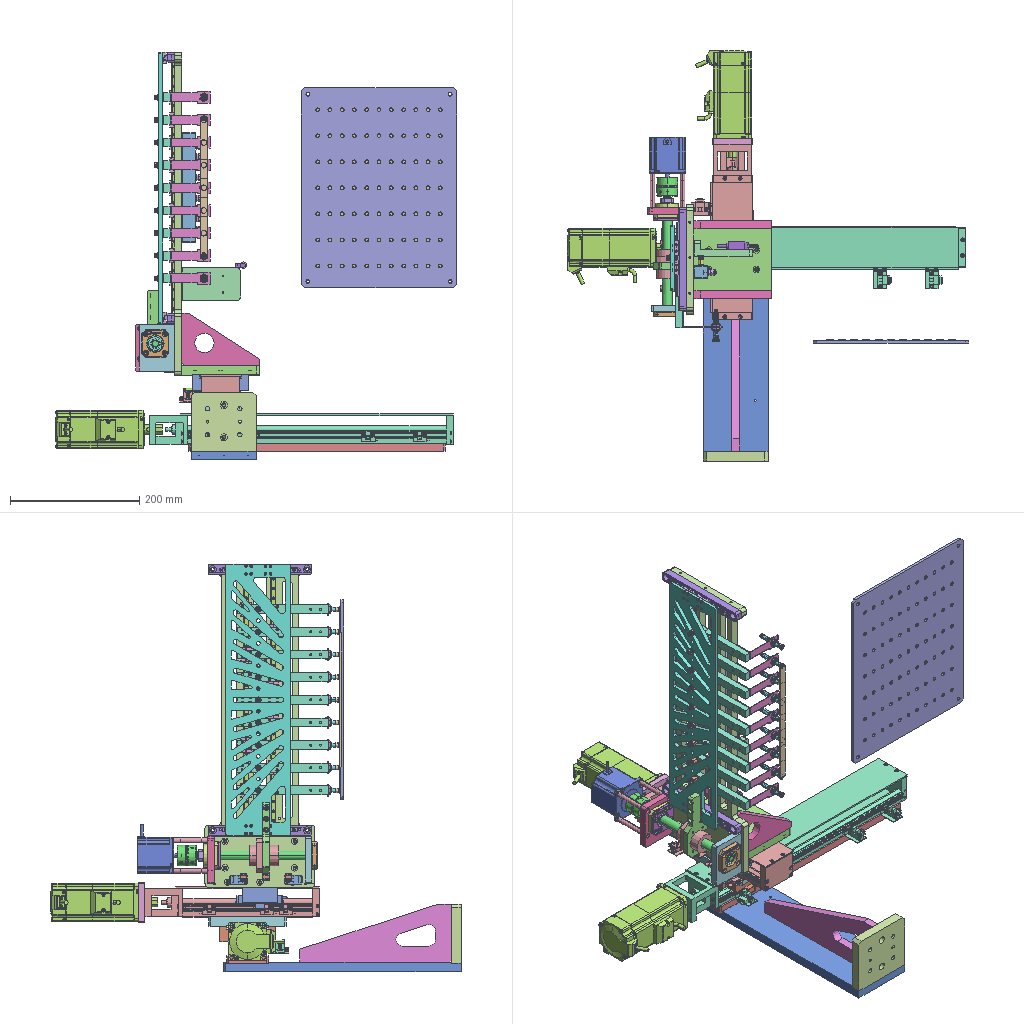Assembly | STEP file | 59 different items | 262 placed | box 621 x 635 x 631 mm
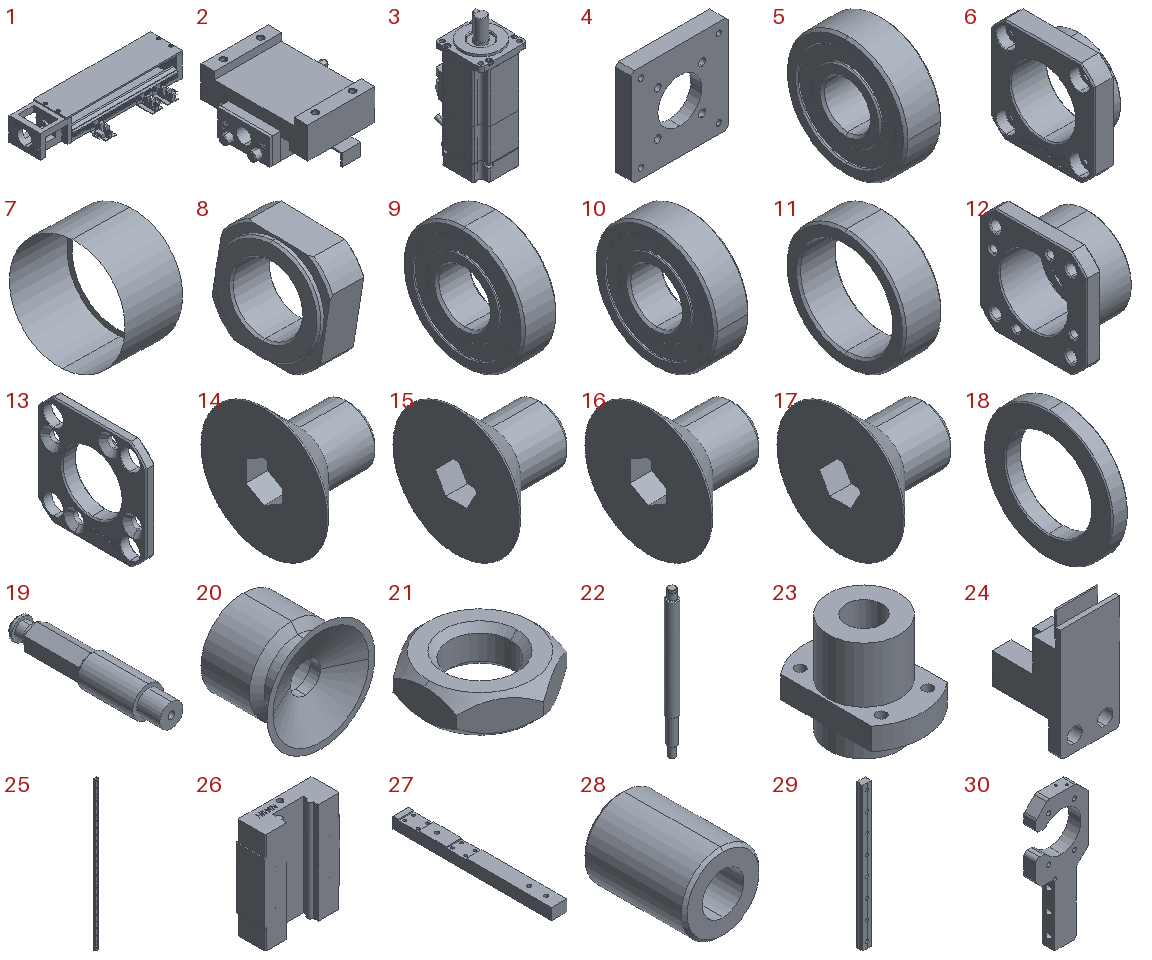Parts list (item | name | quantity | parent item | size | volume):
1 | PRODUCT_ID_1-C-F0-200 | x1 | in KK6005C-200A1-F0CS1-HiwinCorporation-07-20-2018-1 | 270.02 x 94.86 x 47 mm | 309343 mm3
2 | PRODUCT_ID_2-C-F0-200 | x1 | in KK6005C-200A1-F0CS1-HiwinCorporation-07-20-2018-1 | 83.5 x 94 x 36 mm | 123650 mm3
3 | C20604RS (Delta 400W) servo motor | x2 | in KK6005C-200A1-F0CS1-HiwinCorporation-07-20-2018-1, KK6010C-400A1-F0CS1-HiwinCorporation-07-20-2018-1 | 60 x 87.491 x 165.5 mm | 457978 mm3
4 | KK60-F2E KK60 200W flange | x1 | in KK6005C-200A1-F0CS1-HiwinCorporation-07-20-2018-1 | 62 x 10 x 62 mm | 27303 mm3
5 | 6000ZZ-1 | x1 | in LKFF12-1 | 8 x 26 x 26 mm | 3377 mm3
6 | LFF12-1-1 | x1 | in LKFF12-1 | 15 x 42 x 42 mm | 10904 mm3
7 | FANLUOMU19X8X12 | x1 | in 8 | - | -
8 | FANLUOMU19X8X12-1 | x1 | in 8 | 10.153 x 20.245 x 20.375 mm | 1688 mm3
9 | 7001-1 | x1 | in LKFK12-1 | 8 x 28 x 28 mm | 3796 mm3
10 | 7001_1-1 | x1 | in LKFK12-1 | 8 x 28 x 28 mm | 3796 mm3
11 | GELIHUAN15-5-12-1 | x1 | in LKFK12-1 | 5 x 15.5 x 15.5 mm | 371.674 mm3
12 | LFK12-1 | x1 | in LKFK12-1 | 23 x 44 x 44 mm | 14384 mm3
13 | LFK12-GAI-1 | x1 | in LKFK12-1 | 6 x 44 x 44 mm | 4397 mm3
14 | M4-6-1 | x1 | in LKFK12-1 | 6 x 8.819 x 8.819 mm | 121.278 mm3
15 | M4-6_1-1 | x1 | in LKFK12-1 | 6 x 8.819 x 8.819 mm | 121.278 mm3
16 | M4-6_2-1 | x1 | in LKFK12-1 | 6 x 8.819 x 8.819 mm | 121.278 mm3
17 | M4-6_3-1 | x1 | in LKFK12-1 | 6 x 8.819 x 8.819 mm | 121.278 mm3
18 | YOUFENG24X3X16-1 | x1 | in LKFK12-1 | 3 x 24 x 24 mm | 748.955 mm3
19 | PN_0031 | x9 | in PN_0022, PN_0023, PN_0024, PN_0025, PN_0026, PN_0027, PN_0028, PN_0029, PN_0030 | 8 x 40 x 8 mm | 1332 mm3
20 | PN_0033 | x9 | in PN_0022, PN_0023, PN_0024, PN_0025, PN_0026, PN_0027, PN_0028, PN_0029, PN_0030 | 9 x 6.5 x 9 mm | 149.71 mm3
21 | PN_0032 | x18 | in PN_0022, PN_0023, PN_0024, PN_0025, PN_0026, PN_0027, PN_0028, PN_0029, PN_0030 | 12 x 13.856 x 4 mm | 327.385 mm3
22 | HI_LCP02-16-16-L200-F15-P8 | x1 | in LCP02-16-16-L200-F15-P8-1 | 15 x 15 x 200 mm | 29982 mm3
23 | HI_LCP02-16-16-L200-F15-P8_2 | x1 | in LCP02-16-16-L200-F15-P8-1 | 34 x 53 x 45 mm | 34960 mm3
24 | xgSENSOR(EE-SX674) | x2 | in PN_0001 variable-pitch pick-up nozzle-1 | 13.6 x 15.5 x 27.3 mm | 2060 mm3
25 | MGN7C-rail L385 | x2 | in PN_0001 variable-pitch pick-up nozzle-1 | 7 x 4.8 x 385 mm | 11143 mm3
26 | MGN7C-slider block | x13 | in PN_0001 variable-pitch pick-up nozzle-1 | 17 x 6.5 x 22.5 mm | 1844 mm3
27 | PN_0003 | x9 | in PN_0001 variable-pitch pick-up nozzle-1 | 13.5 x 140 x 10 mm | 17518 mm3
28 | PN_0004 | x9 | in PN_0001 variable-pitch pick-up nozzle-1 | 8 x 10.5 x 8 mm | 373.101 mm3
29 | MGN7C-rail L115 | x2 | in PN_0001 variable-pitch pick-up nozzle-1 | 7 x 4.8 x 115 mm | 3319 mm3
30 | PN_0007 | x1 | in PN_0001 variable-pitch pick-up nozzle-1 | 43 x 10 x 110 mm | 21722 mm3
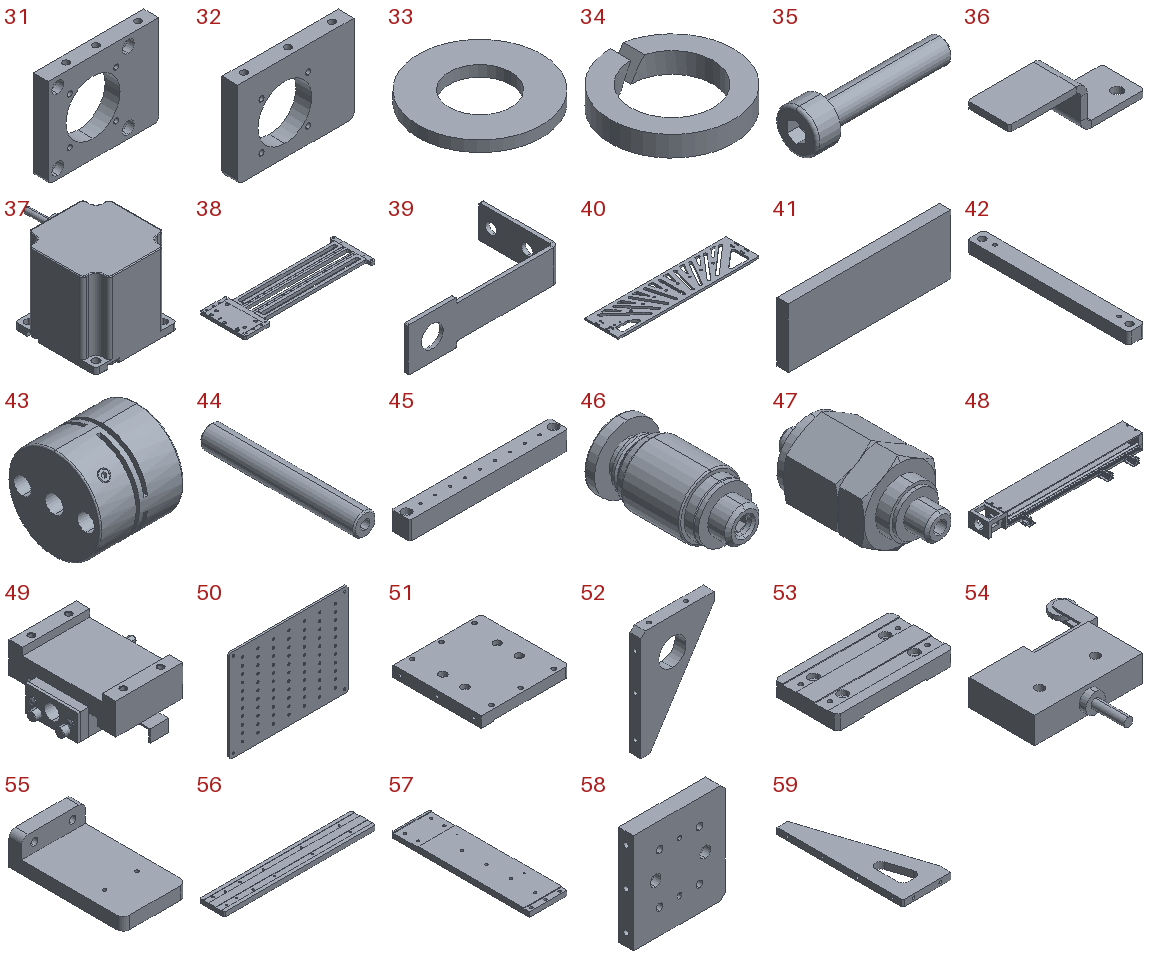31 | PN_0008 | x1 | in PN_0001 variable-pitch pick-up nozzle-1 | 74 x 10 x 60 mm | 31735 mm3
32 | PN_0009 | x1 | in PN_0001 variable-pitch pick-up nozzle-1 | 74 x 10 x 55 mm | 30537 mm3
33 | Flat washer grade C GB T 95-1985 4 | x9 | in PN_0001 variable-pitch pick-up nozzle-1 | 9 x 9 x 0.8 mm | 38.17 mm3
34 | Standard spring lock washer GB T 93-1987 4 | x9 | in PN_0001 variable-pitch pick-up nozzle-1 | 6.6 x 6.6 x 1.1 mm | 20.135 mm3
35 | Hexagon socket head cap screw GB T 70.1-2000 M4X20-C | x9 | in PN_0001 variable-pitch pick-up nozzle-1 | 24 x 7 x 7 mm | 386.251 mm3
36 | PN_0010 (default) | x3 | in PN_0001 variable-pitch pick-up nozzle-1 | 31.5 x 10 x 10 mm | 561.991 mm3
37 | HSTM57-1.8-S-56 | x1 | in PN_0001 variable-pitch pick-up nozzle-1 | 56.438 x 76.419 x 75.6 mm | 160609 mm3
38 | PN_0005 | x1 | in PN_0001 variable-pitch pick-up nozzle-1 | 500 x 170 x 12 mm | 536065 mm3
39 | PN_0011 (default) | x9 | in PN_0001 variable-pitch pick-up nozzle-1 | 62.237 x 31.5 x 18 mm | 1846 mm3
40 | PN_0002 | x1 | in PN_0001 variable-pitch pick-up nozzle-1 | 420 x 100 x 6 mm | 175315 mm3
41 | Part 29.58X10.85X2.08 | x84 | in PN_0001 variable-pitch pick-up nozzle-1, 3. Square aluminium plate (302) - full stock - measured (29.58x10.85x2.08) | 29.58 x 2.08 x 10.85 mm | 667.561 mm3
42 | PN_0006a | x2 | in PN_0001 variable-pitch pick-up nozzle-1 | 16 x 160 x 12 mm | 27789 mm3
43 | DBA01-D32-d6.35-e8 | x1 | in PN_0001 variable-pitch pick-up nozzle-1 | 29 x 32 x 32 mm | 19412 mm3
44 | PN_0012 | x4 | in PN_0001 variable-pitch pick-up nozzle-1 | 8 x 55 x 8 mm | 2556 mm3
45 | PN_0013 | x1 | in PN_0001 variable-pitch pick-up nozzle-1 | 170 x 20 x 20 mm | 64184 mm3
46 | BPOC4M5 | x9 | in PN_0001 variable-pitch pick-up nozzle-1 | 9.5 x 18.5 x 9.5 mm | 733.541 mm3
47 | BKC0425-M3 | x9 | in PN_0001 variable-pitch pick-up nozzle-1 | 8 x 17 x 9.238 mm | 562.812 mm3
48 | PRODUCT_ID_1-C-F0-400 | x1 | in KK6010C-400A1-F0CS1-HiwinCorporation-07-20-2018-1 | 470.02 x 94.86 x 47 mm | 498801 mm3
49 | PRODUCT_ID_2-C-F0-400 | x1 | in KK6010C-400A1-F0CS1-HiwinCorporation-07-20-2018-1 | 83.5 x 94 x 36 mm | 123650 mm3
50 | Square aluminium plate (302) | x1 | in 3. Square aluminium plate (302) - full stock - measured (29.58x10.85x2.08) | 310 x 4.5 x 240 mm | 272267 mm3
51 | PN_0014 | x1 | - | 120 x 120 x 15 mm | 192156 mm3
52 | PN_0015 | x2 | - | 81 x 12 x 120 mm | 60149 mm3
53 | PN_0016 | x1 | - | 120 x 65 x 15 mm | 102204 mm3
54 | Micro switch ZIR52-1703 | x1 | - | 58.94 x 64.5 x 12 mm | 16845 mm3
55 | PN_0021 | x1 | - | 50 x 90 x 25 mm | 51712 mm3
56 | PN_0017 | x1 | - | 398 x 65 x 12 mm | 296877 mm3
57 | PN_0018 | x1 | - | 100 x 368 x 15 mm | 525873 mm3
58 | PN_0019 | x1 | - | 92 x 15 x 100 mm | 130571 mm3
59 | PN_0020 | x1 | - | 90 x 235 x 12 mm | 142926 mm3
Placements (level | parent | child | x y z in mm | rotation matrix by rows):
1 | subassembly 2 | KK6005C-200A1-F0CS1-HiwinCorporation-07-20-2018-1 | 51.0 100.0 60.5 | 0 1 0 -1 0 0 0 0 1
2 | KK6005C-200A1-F0CS1-HiwinCorporation-07-20-2018-1 | PRODUCT_ID_1-C-F0-200 | -0.0 -0.0 -0.0 | 1 0 0 0 1 0 0 0 1
2 | KK6005C-200A1-F0CS1-HiwinCorporation-07-20-2018-1 | PRODUCT_ID_2-C-F0-200 | 19.0 -0.0 -0.0 | 1 0 0 0 1 0 0 0 1
2 | KK6005C-200A1-F0CS1-HiwinCorporation-07-20-2018-1 | C20604RS (Delta 400W) servo motor | -66.0 -0.0 -0.0 | 0 0 1 0 -1 0 1 0 0
2 | KK6005C-200A1-F0CS1-HiwinCorporation-07-20-2018-1 | KK60-F2E KK60 200W flange | -59.0 -0.0 -0.0 | 0 -1 0 1 0 0 0 0 1
1 | subassembly 2 | PN_0001 variable-pitch pick-up nozzle-1 | -246.073 -225.56 374.0 | -1 0 0 0 1 0 0 0 -1
2 | PN_0001 variable-pitch pick-up nozzle-1 | LKFF12-1 | -170.073 118.034 262.0 | 0 -1 0 1 0 0 0 0 1
3 | LKFF12-1 | 6000ZZ-1 | -0.0 0.0 -0.0 | 1 0 0 0 1 0 0 0 1
3 | LKFF12-1 | LFF12-1-1 | -0.0 0.0 -0.0 | 1 0 0 0 1 0 0 0 1
2 | PN_0001 variable-pitch pick-up nozzle-1 | LKFK12-1 | -169.036 271.087 262.954 | 0 -1 0.00171 1 0 0 0 0.00171 1
3 | LKFK12-1 | FANLUOMU19X8X12-1 | 22.348 43.346 2.499 | 0.9935 0.07258 -0.08741 -0.07258 0.9974 0.003182 0.08741 0.003182 0.9962
4 | FANLUOMU19X8X12-1 | FANLUOMU19X8X12 | -0.0 -0.0 -0.0 | 1 0 0 0 1 0 0 0 1
4 | FANLUOMU19X8X12-1 | FANLUOMU19X8X12-1 | -0.0 -0.0 -0.0 | 1 0 0 0 1 0 0 0 1
3 | LKFK12-1 | 7001-1 | -0.0 -0.0 0.0 | 1 0 0 0 1 0 0 0 1
3 | LKFK12-1 | 7001_1-1 | -0.0 -0.0 0.0 | 1 0 0 0 1 0 0 0 1
3 | LKFK12-1 | GELIHUAN15-5-12-1 | 6.641 -31.327 19.206 | 1 0 0 0 1 0 0 0 1
3 | LKFK12-1 | LFK12-1 | -0.0 -0.0 0.0 | 1 0 0 0 1 0 0 0 1
3 | LKFK12-1 | LFK12-GAI-1 | -0.0 -0.0 0.0 | 1 0 0 0 1 0 0 0 1
3 | LKFK12-1 | M4-6-1 | -0.0 -0.0 0.0 | 1 0 0 0 1 0 0 0 1
3 | LKFK12-1 | M4-6_1-1 | -0.0 -0.0 0.0 | 1 0 0 0 1 0 0 0 1
3 | LKFK12-1 | M4-6_2-1 | -0.0 -0.0 0.0 | 1 0 0 0 1 0 0 0 1
3 | LKFK12-1 | M4-6_3-1 | -0.0 -0.0 0.0 | 1 0 0 0 1 0 0 0 1
3 | LKFK12-1 | YOUFENG24X3X16-1 | -0.0 -0.0 0.0 | 1 0 0 0 1 0 0 0 1
2 | PN_0001 variable-pitch pick-up nozzle-1 | PN_0022 | -271.31 102.59 140.076 | 1 0 0 0 1 0 0 0 1
3 | PN_0022 | PN_0031 | -0.0 -13.5 -0.0 | 1 0 0 0 1 0 0 0 1
3 | PN_0022 | PN_0033 | -0.0 -13.5 -0.0 | 1 0 0 0 1 0 0 0 1
3 | PN_0022 | PN_0032 | 0.0 -1.5 0.0 | 1 0 0 0 0 -1 0 1 0
3 | PN_0022 | PN_0032 | 0.0 -0.0 0.0 | 1 0 0 0 0 1 0 -1 0
2 | PN_0001 variable-pitch pick-up nozzle-1 | PN_0023 | -271.31 102.59 105.066 | 1 0 0 0 1 0 0 0 1
3 | PN_0023 | PN_0031 | -0.0 -13.5 0.0 | 1 0 0 0 1 0 0 0 1
3 | PN_0023 | PN_0033 | -0.0 -13.5 0.0 | 1 0 0 0 1 0 0 0 1
3 | PN_0023 | PN_0032 | 0.0 -0.0 0.0 | 1 0 0 0 0 1 0 -1 0
3 | PN_0023 | PN_0032 | 0.0 -1.5 0.0 | 1 0 0 0 0 -1 0 1 0
2 | PN_0001 variable-pitch pick-up nozzle-1 | PN_0024 | -271.31 102.59 70.058 | 1 0 0 0 1 0 0 0 1
3 | PN_0024 | PN_0031 | -0.0 -13.5 0.0 | 1 0 0 0 1 0 0 0 1
3 | PN_0024 | PN_0033 | -0.0 -13.5 0.0 | 1 0 0 0 1 0 0 0 1
3 | PN_0024 | PN_0032 | 0.0 -1.5 0.0 | 1 0 0 0 0 -1 0 1 0
3 | PN_0024 | PN_0032 | 0.0 -0.0 0.0 | 1 0 0 0 0 1 0 -1 0
2 | PN_0001 variable-pitch pick-up nozzle-1 | PN_0025 | -271.31 102.59 35.052 | 1 0 0 0 1 0 0 0 1
3 | PN_0025 | PN_0031 | -0.0 -13.5 0.0 | 1 0 0 0 1 0 0 0 1
3 | PN_0025 | PN_0033 | -0.0 -13.5 0.0 | 1 0 0 0 1 0 0 0 1
3 | PN_0025 | PN_0032 | 0.0 -1.5 0.0 | 1 0 0 0 0 -1 0 1 0
3 | PN_0025 | PN_0032 | 0.0 -0.0 0.0 | 1 0 0 0 0 1 0 -1 0
2 | PN_0001 variable-pitch pick-up nozzle-1 | PN_0026 | -271.31 102.59 0.0 | -0.07822 0 0.9969 0 1 0 -0.9969 0 -0.07822
3 | PN_0026 | PN_0031 | -0.0 -13.5 -0.0 | 1 0 0 0 1 0 0 0 1
3 | PN_0026 | PN_0033 | -0.0 -13.5 -0.0 | 1 0 0 0 1 0 0 0 1
3 | PN_0026 | PN_0032 | -0.0 -1.5 -0.0 | 1 0 0 0 0 -1 0 1 0
3 | PN_0026 | PN_0032 | -0.0 -0.0 -0.0 | 1 0 0 0 0 1 0 -1 -0
2 | PN_0001 variable-pitch pick-up nozzle-1 | PN_0027 | -271.31 102.59 -35.052 | 1 0 0 0 1 0 0 0 1
3 | PN_0027 | PN_0031 | -0.0 -13.5 0.0 | 1 0 0 0 1 0 0 0 1
3 | PN_0027 | PN_0033 | -0.0 -13.5 0.0 | 1 0 0 0 1 0 0 0 1
3 | PN_0027 | PN_0032 | 0.0 -0.0 0.0 | 1 0 0 0 0 1 0 -1 0
3 | PN_0027 | PN_0032 | 0.0 -1.5 0.0 | 1 0 0 0 0 -1 0 1 0
2 | PN_0001 variable-pitch pick-up nozzle-1 | PN_0028 | -271.31 102.59 -70.058 | 1 0 0 0 1 0 0 0 1
3 | PN_0028 | PN_0031 | -0.0 -13.5 0.0 | 1 0 0 0 1 0 0 0 1
3 | PN_0028 | PN_0033 | -0.0 -13.5 0.0 | 1 0 0 0 1 0 0 0 1
3 | PN_0028 | PN_0032 | 0.0 -1.5 0.0 | 1 0 0 0 0 -1 0 1 0
3 | PN_0028 | PN_0032 | 0.0 -0.0 0.0 | 1 0 0 0 0 1 0 -1 0
2 | PN_0001 variable-pitch pick-up nozzle-1 | PN_0029 | -271.31 102.59 -140.076 | 0.9981 0 0.06111 0 1 0 -0.06111 0 0.9981
3 | PN_0029 | PN_0031 | -0.0 -13.5 -0.0 | 1 0 0 0 1 0 0 0 1
3 | PN_0029 | PN_0033 | -0.0 -13.5 -0.0 | 1 0 0 0 1 0 0 0 1
3 | PN_0029 | PN_0032 | -0.0 -1.5 -0.0 | 1 0 0 0 0 -1 0 1 0
3 | PN_0029 | PN_0032 | -0.0 -0.0 -0.0 | 1 0 0 0 0 1 0 -1 -0
2 | PN_0001 variable-pitch pick-up nozzle-1 | PN_0030 | -271.31 102.59 -105.066 | 1 0 0 0 1 0 0 0 1
3 | PN_0030 | PN_0031 | -0.0 -13.5 0.0 | 1 0 0 0 1 0 0 0 1
3 | PN_0030 | PN_0033 | -0.0 -13.5 0.0 | 1 0 0 0 1 0 0 0 1
3 | PN_0030 | PN_0032 | 0.0 -1.5 0.0 | 1 0 0 0 0 -1 0 1 0
3 | PN_0030 | PN_0032 | 0.0 -0.0 0.0 | 1 0 0 0 0 1 0 -1 0
2 | PN_0001 variable-pitch pick-up nozzle-1 | LCP02-16-16-L200-F15-P8-1 | -196.073 118.493 241.0 | 1 0 0 0 0 -1 0 1 -0
3 | LCP02-16-16-L200-F15-P8-1 | HI_LCP02-16-16-L200-F15-P8 | -0.0 0.0 0.0 | 1 0 0 0 1 0 0 0 1
3 | LCP02-16-16-L200-F15-P8-1 | HI_LCP02-16-16-L200-F15-P8_2 | -0.0 0.0 0.0 | 1 0 0 0 1 0 0 0 1
2 | PN_0001 variable-pitch pick-up nozzle-1 | xgSENSOR(EE-SX674) | -225.073 247.393 278.25 | 0 1 0 0 0 1 1 0 0
2 | PN_0001 variable-pitch pick-up nozzle-1 | xgSENSOR(EE-SX674) | -225.073 146.393 278.25 | 0 1 0 0 0 -1 -1 0 -0
2 | PN_0001 variable-pitch pick-up nozzle-1 | MGN7C-rail L385 | -226.073 185.53 -172.5 | 0 1 0 -1 0 0 0 0 1
2 | PN_0001 variable-pitch pick-up nozzle-1 | MGN7C-rail L385 | -226.073 227.59 -172.5 | 0 1 0 -1 0 0 0 0 1
2 | PN_0001 variable-pitch pick-up nozzle-1 | MGN7C-slider block | -214.573 224.04 -201.0 | 0 1 0 0 0 -1 -1 0 -0
2 | PN_0001 variable-pitch pick-up nozzle-1 | MGN7C-slider block | -226.073 227.59 -0.0 | 0 1 0 -1 0 0 0 0 1
2 | PN_0001 variable-pitch pick-up nozzle-1 | MGN7C-slider block | -214.573 194.04 201.0 | 0 1 0 0 0 -1 -1 0 -0
2 | PN_0001 variable-pitch pick-up nozzle-1 | MGN7C-slider block | -226.073 227.59 -70.058 | 0 1 0 -1 0 0 0 0 1
2 | PN_0001 variable-pitch pick-up nozzle-1 | MGN7C-slider block | -214.573 194.04 -201.0 | 0 1 0 0 0 -1 -1 0 -0
2 | PN_0001 variable-pitch pick-up nozzle-1 | MGN7C-slider block | -226.073 185.53 105.066 | 0 1 0 -1 0 0 0 0 1
2 | PN_0001 variable-pitch pick-up nozzle-1 | MGN7C-slider block | -226.073 227.59 -140.076 | 0 1 0 -1 0 0 0 0 1
2 | PN_0001 variable-pitch pick-up nozzle-1 | MGN7C-slider block | -226.073 185.53 35.052 | 0 1 0 -1 0 0 0 0 1
2 | PN_0001 variable-pitch pick-up nozzle-1 | MGN7C-slider block | -226.073 227.59 70.058 | 0 1 0 -1 0 0 0 0 1
2 | PN_0001 variable-pitch pick-up nozzle-1 | MGN7C-slider block | -226.073 185.53 -35.052 | 0 1 0 -1 0 0 0 0 1
2 | PN_0001 variable-pitch pick-up nozzle-1 | MGN7C-slider block | -226.073 227.59 140.076 | 0 1 0 -1 0 0 0 0 1
2 | PN_0001 variable-pitch pick-up nozzle-1 | MGN7C-slider block | -226.073 185.53 -105.066 | 0 1 0 -1 0 0 0 0 1
2 | PN_0001 variable-pitch pick-up nozzle-1 | MGN7C-slider block | -214.573 224.04 201.0 | 0 1 0 0 0 -1 -1 0 -0
2 | PN_0001 variable-pitch pick-up nozzle-1 | PN_0003 | -214.073 171.09 35.052 | 0 0 -1 0 1 0 1 0 0
2 | PN_0001 variable-pitch pick-up nozzle-1 | PN_0003 | -214.073 171.09 -35.052 | 0 0 -1 0 1 0 1 0 0
2 | PN_0001 variable-pitch pick-up nozzle-1 | PN_0003 | -214.073 171.09 -105.066 | 0 0 -1 0 1 0 1 0 0
2 | PN_0001 variable-pitch pick-up nozzle-1 | PN_0003 | -214.073 171.09 70.058 | 0 0 -1 0 1 0 1 0 0
2 | PN_0001 variable-pitch pick-up nozzle-1 | PN_0003 | -214.073 171.09 140.076 | 0 0 -1 0 1 0 1 0 0
2 | PN_0001 variable-pitch pick-up nozzle-1 | PN_0003 | -214.073 171.09 105.066 | 0 0 -1 0 1 0 1 0 0
2 | PN_0001 variable-pitch pick-up nozzle-1 | PN_0003 | -214.073 171.09 -0.0 | 0 0 -1 0 1 0 1 0 0
2 | PN_0001 variable-pitch pick-up nozzle-1 | PN_0003 | -214.073 171.09 -70.058 | 0 0 -1 0 1 0 1 0 0
2 | PN_0001 variable-pitch pick-up nozzle-1 | PN_0003 | -214.073 171.09 -140.076 | 0 0 -1 0 1 0 1 0 0
2 | PN_0001 variable-pitch pick-up nozzle-1 | PN_0004 | -205.323 209.04 35.052 | 0 1 0 -0.201 0 0.9796 0.9796 0 0.201
2 | PN_0001 variable-pitch pick-up nozzle-1 | PN_0004 | -205.323 209.04 -0.0 | 0 1 0 -0.5153 0 0.857 0.857 0 0.5153
2 | PN_0001 variable-pitch pick-up nozzle-1 | PN_0004 | -205.323 209.04 -70.058 | 0 1 0 -0.4151 0 0.9098 0.9098 0 0.4151
2 | PN_0001 variable-pitch pick-up nozzle-1 | PN_0004 | -205.323 209.04 -140.076 | 0 1 0 -0.5153 0 0.857 0.857 0 0.5153
2 | PN_0001 variable-pitch pick-up nozzle-1 | PN_0004 | -205.323 209.04 -105.066 | 0 1 0 -0.4151 0 0.9098 0.9098 0 0.4151
2 | PN_0001 variable-pitch pick-up nozzle-1 | PN_0004 | -205.323 209.04 140.076 | 0 1 0 0.4098 0 -0.9122 -0.9122 0 -0.4098
2 | PN_0001 variable-pitch pick-up nozzle-1 | PN_0004 | -205.323 209.04 105.066 | 0 1 0 0.8533 0 -0.5214 -0.5214 0 -0.8533
2 | PN_0001 variable-pitch pick-up nozzle-1 | PN_0004 | -205.323 209.04 -35.052 | 0 -1 0 -0.9888 0 -0.149 0.149 0 -0.9888
2 | PN_0001 variable-pitch pick-up nozzle-1 | PN_0004 | -205.323 209.04 70.058 | 0 1 0 -0.201 0 0.9796 0.9796 0 0.201
2 | PN_0001 variable-pitch pick-up nozzle-1 | MGN7C-rail L115 | -214.573 244.06 201.0 | 0 1 0 0 0 -1 -1 0 -0
2 | PN_0001 variable-pitch pick-up nozzle-1 | MGN7C-rail L115 | -214.573 244.06 -201.0 | 0 1 0 0 0 -1 -1 0 -0
2 | PN_0001 variable-pitch pick-up nozzle-1 | PN_0007 | -196.073 201.893 241.0 | 1 0 0 0 1 0 0 0 1
2 | PN_0001 variable-pitch pick-up nozzle-1 | PN_0008 | -196.073 277.087 248.0 | 0 0 -1 0 1 0 1 0 -0
2 | PN_0001 variable-pitch pick-up nozzle-1 | PN_0009 | -198.573 126.034 248.0 | 0 0 -1 0 1 0 1 0 -0
2 | PN_0001 variable-pitch pick-up nozzle-1 | Flat washer grade C GB T 95-1985 4 | -200.073 209.04 -35.052 | 0 0 -1 -0.7058 0.7084 0 0.7084 0.7058 -0
2 | PN_0001 variable-pitch pick-up nozzle-1 | Flat washer grade C GB T 95-1985 4 | -200.073 209.04 -140.076 | 0 0 -1 -0.9242 -0.3818 0 -0.3818 0.9242 0
2 | PN_0001 variable-pitch pick-up nozzle-1 | Flat washer grade C GB T 95-1985 4 | -200.073 209.04 70.058 | 0 0 -1 0.7058 -0.7084 0 -0.7084 -0.7058 0
2 | PN_0001 variable-pitch pick-up nozzle-1 | Flat washer grade C GB T 95-1985 4 | -199.273 209.04 140.076 | 0 0 1 0 1 0 -1 0 -0
2 | PN_0001 variable-pitch pick-up nozzle-1 | Flat washer grade C GB T 95-1985 4 | -200.073 209.04 35.052 | 0 0 -1 -0.9242 -0.3818 0 -0.3818 0.9242 0
2 | PN_0001 variable-pitch pick-up nozzle-1 | Flat washer grade C GB T 95-1985 4 | -200.073 209.04 0.0 | 0 0 -1 -0.7058 0.7084 0 0.7084 0.7058 0
2 | PN_0001 variable-pitch pick-up nozzle-1 | Flat washer grade C GB T 95-1985 4 | -200.073 209.04 -105.066 | 0 0 -1 -0.7058 0.7084 0 0.7084 0.7058 0
2 | PN_0001 variable-pitch pick-up nozzle-1 | Flat washer grade C GB T 95-1985 4 | -200.073 209.04 105.066 | 0 0 -1 -0.9242 -0.3818 0 -0.3818 0.9242 0
2 | PN_0001 variable-pitch pick-up nozzle-1 | Flat washer grade C GB T 95-1985 4 | -200.073 209.04 -70.058 | 0 0 -1 -0.7058 0.7084 0 0.7084 0.7058 -0
2 | PN_0001 variable-pitch pick-up nozzle-1 | Standard spring lock washer GB T 93-1987 4 | -199.273 209.04 105.066 | 0 0 -1 0 1 0 1 0 0
2 | PN_0001 variable-pitch pick-up nozzle-1 | Standard spring lock washer GB T 93-1987 4 | -199.273 209.04 -140.076 | 0 0 -1 -0.236 -0.9718 0 -0.9718 0.236 0
2 | PN_0001 variable-pitch pick-up nozzle-1 | Standard spring lock washer GB T 93-1987 4 | -199.273 209.04 70.058 | 0 0 -1 0.9242 0.3818 0 0.3818 -0.9242 0
2 | PN_0001 variable-pitch pick-up nozzle-1 | Standard spring lock washer GB T 93-1987 4 | -199.273 209.04 35.052 | 0 0 -1 0.9242 0.3818 0 0.3818 -0.9242 0
2 | PN_0001 variable-pitch pick-up nozzle-1 | Standard spring lock washer GB T 93-1987 4 | -198.173 209.04 140.076 | 0 0 1 0 1 0 -1 0 -0
2 | PN_0001 variable-pitch pick-up nozzle-1 | Standard spring lock washer GB T 93-1987 4 | -199.273 209.04 0.0 | 0 0 -1 0.9242 0.3818 0 0.3818 -0.9242 -0
2 | PN_0001 variable-pitch pick-up nozzle-1 | Standard spring lock washer GB T 93-1987 4 | -199.273 209.04 -105.066 | 0 0 -1 -0.9882 -0.1529 0 -0.1529 0.9882 0
2 | PN_0001 variable-pitch pick-up nozzle-1 | Standard spring lock washer GB T 93-1987 4 | -199.273 209.04 -70.058 | 0 0 -1 -0.9882 -0.1529 0 -0.1529 0.9882 -0
2 | PN_0001 variable-pitch pick-up nozzle-1 | Standard spring lock washer GB T 93-1987 4 | -199.273 209.04 -35.052 | 0 0 -1 0.9242 0.3818 0 0.3818 -0.9242 0
2 | PN_0001 variable-pitch pick-up nozzle-1 | Hexagon socket head cap screw GB T 70.1-2000 M4X20-C | -194.173 209.04 -140.076 | -1 0 0 0 -0.3818 0.9242 0 0.9242 0.3818
2 | PN_0001 variable-pitch pick-up nozzle-1 | Hexagon socket head cap screw GB T 70.1-2000 M4X20-C | -194.173 209.04 70.058 | -1 0 0 0 -0.3818 0.9242 0 0.9242 0.3818
2 | PN_0001 variable-pitch pick-up nozzle-1 | Hexagon socket head cap screw GB T 70.1-2000 M4X20-C | -194.173 209.04 105.066 | -1 0 0 0 -0.7966 0.6046 0 0.6046 0.7966
2 | PN_0001 variable-pitch pick-up nozzle-1 | Hexagon socket head cap screw GB T 70.1-2000 M4X20-C | -194.173 209.04 140.076 | -1 0 0 0 -0.3818 0.9242 0 0.9242 0.3818
2 | PN_0001 variable-pitch pick-up nozzle-1 | Hexagon socket head cap screw GB T 70.1-2000 M4X20-C | -194.173 209.04 -0.0 | -1 0 0 0 -0.3818 0.9242 0 0.9242 0.3818
2 | PN_0001 variable-pitch pick-up nozzle-1 | Hexagon socket head cap screw GB T 70.1-2000 M4X20-C | -194.173 209.04 -105.066 | -1 0 0 0 -0.9864 0.1646 0 0.1646 0.9864
2 | PN_0001 variable-pitch pick-up nozzle-1 | Hexagon socket head cap screw GB T 70.1-2000 M4X20-C | -194.173 209.04 35.052 | -1 0 0 0 -0.3818 0.9242 0 0.9242 0.3818
2 | PN_0001 variable-pitch pick-up nozzle-1 | Hexagon socket head cap screw GB T 70.1-2000 M4X20-C | -194.173 209.04 -70.058 | -1 0 0 0 -0.9864 0.1646 0 0.1646 0.9864
2 | PN_0001 variable-pitch pick-up nozzle-1 | Hexagon socket head cap screw GB T 70.1-2000 M4X20-C | -194.173 209.04 -35.052 | -1 0 0 0 0.9242 0.3818 0 0.3818 -0.9242
2 | PN_0001 variable-pitch pick-up nozzle-1 | PN_0010 (default) | -200.073 196.893 270.5 | 1 0 0 0 1 0 0 0 1
2 | PN_0001 variable-pitch pick-up nozzle-1 | PN_0010 (default) | -200.073 231.893 270.5 | 1 0 0 0 1 0 0 0 1
2 | PN_0001 variable-pitch pick-up nozzle-1 | PN_0010 (default) | -200.073 161.893 270.5 | 1 0 0 0 1 0 0 0 1
2 | PN_0001 variable-pitch pick-up nozzle-1 | HSTM57-1.8-S-56 | -196.073 356.087 241.0 | 1 0 0 0 0 1 0 -1 0
2 | PN_0001 variable-pitch pick-up nozzle-1 | PN_0005 | -231.073 206.56 -0.0 | 0 0 1 0 1 0 -1 0 0
2 | PN_0001 variable-pitch pick-up nozzle-1 | PN_0011 (default) | -251.31 102.59 35.052 | 1 0 0 0 1 0 0 0 1
2 | PN_0001 variable-pitch pick-up nozzle-1 | PN_0011 (default) | -251.31 102.59 140.076 | 1 0 0 0 1 0 0 0 1
2 | PN_0001 variable-pitch pick-up nozzle-1 | PN_0011 (default) | -251.31 102.59 -70.058 | 1 0 0 0 1 0 0 0 1
2 | PN_0001 variable-pitch pick-up nozzle-1 | PN_0011 (default) | -251.31 102.59 0.0 | 1 0 0 0 1 0 0 0 1
2 | PN_0001 variable-pitch pick-up nozzle-1 | PN_0011 (default) | -251.31 102.59 -140.076 | 1 0 0 0 1 0 0 0 1
2 | PN_0001 variable-pitch pick-up nozzle-1 | PN_0011 (default) | -251.31 102.59 70.058 | 1 0 0 0 1 0 0 0 1
2 | PN_0001 variable-pitch pick-up nozzle-1 | PN_0011 (default) | -251.31 102.59 -105.066 | 1 0 0 0 1 0 0 0 1
2 | PN_0001 variable-pitch pick-up nozzle-1 | PN_0011 (default) | -251.31 102.59 -35.052 | 1 0 0 0 1 0 0 0 1
2 | PN_0001 variable-pitch pick-up nozzle-1 | PN_0011 (default) | -251.31 102.59 105.066 | 1 0 0 0 1 0 0 0 1
2 | PN_0001 variable-pitch pick-up nozzle-1 | PN_0002 | -204.573 209.04 0.0 | 0 0 1 0 1 0 -1 0 -0
2 | PN_0001 variable-pitch pick-up nozzle-1 | Part 29.58X10.85X2.08 | -271.31 81.55 -88.8 | 0 0 -1 0 1 0 1 0 0
2 | PN_0001 variable-pitch pick-up nozzle-1 | Part 29.58X10.85X2.08 | -271.31 81.55 88.8 | 0 0 -1 0 1 0 1 0 0
2 | PN_0001 variable-pitch pick-up nozzle-1 | Part 29.58X10.85X2.08 | -271.31 81.55 59.2 | 0 0 -1 0 1 0 1 0 0
2 | PN_0001 variable-pitch pick-up nozzle-1 | Part 29.58X10.85X2.08 | -271.31 81.55 29.6 | 0 0 -1 0 1 0 1 0 0
2 | PN_0001 variable-pitch pick-up nozzle-1 | Part 29.58X10.85X2.08 | -271.31 81.55 -0.0 | 0 0 -1 0 1 0 1 0 0
2 | PN_0001 variable-pitch pick-up nozzle-1 | Part 29.58X10.85X2.08 | -271.31 81.55 -29.6 | 0 0 -1 0 1 0 1 0 0
2 | PN_0001 variable-pitch pick-up nozzle-1 | Part 29.58X10.85X2.08 | -271.31 81.55 -59.2 | 0 0 -1 0 1 0 1 0 0
2 | PN_0001 variable-pitch pick-up nozzle-1 | PN_0006a | -220.073 206.56 202.0 | 0 0 -1 0 -1 0 -1 0 -0
2 | PN_0001 variable-pitch pick-up nozzle-1 | PN_0006a | -220.073 206.56 -202.0 | 0 0 -1 0 1 0 1 0 -0
2 | PN_0001 variable-pitch pick-up nozzle-1 | DBA01-D32-d6.35-e8 | -196.073 319.687 241.0 | 0 0.9985 0.05439 -1 0 0 0 -0.05439 0.9985
2 | PN_0001 variable-pitch pick-up nozzle-1 | PN_0012 | -172.503 313.587 264.57 | 1 0 0 0 1 0 0 0 1
2 | PN_0001 variable-pitch pick-up nozzle-1 | PN_0012 | -219.645 313.587 264.571 | 1 0 0 0 1 0 0 0 1
2 | PN_0001 variable-pitch pick-up nozzle-1 | PN_0012 | -219.643 313.587 217.43 | 1 0 0 0 1 0 0 0 1
2 | PN_0001 variable-pitch pick-up nozzle-1 | PN_0012 | -172.503 313.587 217.43 | 1 0 0 0 1 0 0 0 1
2 | PN_0001 variable-pitch pick-up nozzle-1 | PN_0013 | -248.073 186.56 -0.0 | 0 0 -1 0 1 0 1 0 -0
2 | PN_0001 variable-pitch pick-up nozzle-1 | BPOC4M5 | -248.073 193.66 48.0 | 1 0 0 0 1 0 0 0 1
2 | PN_0001 variable-pitch pick-up nozzle-1 | BPOC4M5 | -248.073 193.66 64.0 | 1 0 0 0 1 0 0 0 1
2 | PN_0001 variable-pitch pick-up nozzle-1 | BPOC4M5 | -248.073 193.66 -48.0 | 1 0 0 0 1 0 0 0 1
2 | PN_0001 variable-pitch pick-up nozzle-1 | BPOC4M5 | -248.073 193.66 -32.0 | 1 0 0 0 1 0 0 0 1
2 | PN_0001 variable-pitch pick-up nozzle-1 | BPOC4M5 | -248.073 193.66 -16.0 | 1 0 0 0 1 0 0 0 1
2 | PN_0001 variable-pitch pick-up nozzle-1 | BPOC4M5 | -248.073 193.66 -0.0 | 1 0 0 0 1 0 0 0 1
2 | PN_0001 variable-pitch pick-up nozzle-1 | BPOC4M5 | -248.073 193.66 16.0 | 1 0 0 0 1 0 0 0 1
2 | PN_0001 variable-pitch pick-up nozzle-1 | BPOC4M5 | -248.073 193.66 -64.0 | 1 0 0 0 1 0 0 0 1
2 | PN_0001 variable-pitch pick-up nozzle-1 | BPOC4M5 | -248.073 193.66 32.0 | 1 0 0 0 1 0 0 0 1
2 | PN_0001 variable-pitch pick-up nozzle-1 | BKC0425-M3 | -255.473 186.56 -64.0 | 0 -1 0 -0.3818 0 -0.9242 0.9242 0 -0.3818
2 | PN_0001 variable-pitch pick-up nozzle-1 | BKC0425-M3 | -255.473 186.56 -48.0 | 0 -1 0 -0.3818 0 -0.9242 0.9242 0 -0.3818
2 | PN_0001 variable-pitch pick-up nozzle-1 | BKC0425-M3 | -255.473 186.56 -32.0 | 0 -1 0 -0.3818 0 -0.9242 0.9242 0 -0.3818
2 | PN_0001 variable-pitch pick-up nozzle-1 | BKC0425-M3 | -255.473 186.56 64.0 | 0 -1 0 -0.3818 0 -0.9242 0.9242 0 -0.3818
2 | PN_0001 variable-pitch pick-up nozzle-1 | BKC0425-M3 | -255.473 186.56 -16.0 | 0 -1 0 -0.3818 0 -0.9242 0.9242 0 -0.3818
2 | PN_0001 variable-pitch pick-up nozzle-1 | BKC0425-M3 | -255.473 186.56 -0.0 | 0 -1 0 -0.3818 0 -0.9242 0.9242 0 -0.3818
2 | PN_0001 variable-pitch pick-up nozzle-1 | BKC0425-M3 | -255.473 186.56 16.0 | 0 -1 0 -0.3818 0 -0.9242 0.9242 0 -0.3818
2 | PN_0001 variable-pitch pick-up nozzle-1 | BKC0425-M3 | -255.473 186.56 48.0 | 0 -1 0 -0.3818 0 -0.9242 0.9242 0 -0.3818
2 | PN_0001 variable-pitch pick-up nozzle-1 | BKC0425-M3 | -255.473 186.56 32.0 | 0 -1 0 -0.3818 0 -0.9242 0.9242 0 -0.3818
1 | subassembly 2 | KK6010C-400A1-F0CS1-HiwinCorporation-07-20-2018-1 | -0.0 -0.0 -0.0 | 1 0 0 0 1 0 0 0 1
2 | KK6010C-400A1-F0CS1-HiwinCorporation-07-20-2018-1 | C20604RS (Delta 400W) servo motor | -66.0 -0.0 -0.0 | 0 0 1 0 -1 0 1 0 0
2 | KK6010C-400A1-F0CS1-HiwinCorporation-07-20-2018-1 | PRODUCT_ID_1-C-F0-400 | -0.0 -0.0 -0.0 | 1 0 0 0 1 0 0 0 1
2 | KK6010C-400A1-F0CS1-HiwinCorporation-07-20-2018-1 | PRODUCT_ID_2-C-F0-400 | -149.0 -0.0 -0.0 | 1 0 0 0 1 0 0 0 1
1 | subassembly 2 | 3. Square aluminium plate (302) - full stock - measured (29.58x10.85x2.08) | 296.237 -148.55 374.0 | 0 0 1 0 1 0 -1 0 0
2 | 3. Square aluminium plate (302) - full stock - measured (29.58x10.85x2.08) | Part 29.58X10.85X2.08 | -0.0 4.54 -76.0 | 1 0 0 0 1 0 0 0 1
2 | 3. Square aluminium plate (302) - full stock - measured (29.58x10.85x2.08) | Part 29.58X10.85X2.08 | -120.9 4.54 76.0 | 1 0 0 0 1 0 0 0 1
2 | 3. Square aluminium plate (302) - full stock - measured (29.58x10.85x2.08) | Part 29.58X10.85X2.08 | 120.9 4.54 19.0 | 1 0 0 0 1 0 0 0 1
2 | 3. Square aluminium plate (302) - full stock - measured (29.58x10.85x2.08) | Part 29.58X10.85X2.08 | 40.3 4.54 -38.0 | 1 0 0 0 1 0 0 0 1
2 | 3. Square aluminium plate (302) - full stock - measured (29.58x10.85x2.08) | Part 29.58X10.85X2.08 | -40.3 4.54 -95.0 | 1 0 0 0 1 0 0 0 1
2 | 3. Square aluminium plate (302) - full stock - measured (29.58x10.85x2.08) | Part 29.58X10.85X2.08 | 80.6 4.54 -0.0 | 1 0 0 0 1 0 0 0 1
2 | 3. Square aluminium plate (302) - full stock - measured (29.58x10.85x2.08) | Part 29.58X10.85X2.08 | -0.0 4.54 -57.0 | 1 0 0 0 1 0 0 0 1
2 | 3. Square aluminium plate (302) - full stock - measured (29.58x10.85x2.08) | Part 29.58X10.85X2.08 | -120.9 4.54 95.0 | 1 0 0 0 1 0 0 0 1
2 | 3. Square aluminium plate (302) - full stock - measured (29.58x10.85x2.08) | Part 29.58X10.85X2.08 | 120.9 4.54 38.0 | 1 0 0 0 1 0 0 0 1
2 | 3. Square aluminium plate (302) - full stock - measured (29.58x10.85x2.08) | Part 29.58X10.85X2.08 | 40.3 4.54 -19.0 | 1 0 0 0 1 0 0 0 1
2 | 3. Square aluminium plate (302) - full stock - measured (29.58x10.85x2.08) | Part 29.58X10.85X2.08 | -40.3 4.54 -76.0 | 1 0 0 0 1 0 0 0 1
2 | 3. Square aluminium plate (302) - full stock - measured (29.58x10.85x2.08) | Part 29.58X10.85X2.08 | 80.6 4.54 19.0 | 1 0 0 0 1 0 0 0 1
2 | 3. Square aluminium plate (302) - full stock - measured (29.58x10.85x2.08) | Part 29.58X10.85X2.08 | 0.0 4.54 -38.0 | 1 0 0 0 1 0 0 0 1
2 | 3. Square aluminium plate (302) - full stock - measured (29.58x10.85x2.08) | Part 29.58X10.85X2.08 | -80.6 4.54 -95.0 | 1 0 0 0 1 0 0 0 1
2 | 3. Square aluminium plate (302) - full stock - measured (29.58x10.85x2.08) | Part 29.58X10.85X2.08 | 120.9 4.54 57.0 | 1 0 0 0 1 0 0 0 1
2 | 3. Square aluminium plate (302) - full stock - measured (29.58x10.85x2.08) | Part 29.58X10.85X2.08 | 40.3 4.54 -0.0 | 1 0 0 0 1 0 0 0 1
2 | 3. Square aluminium plate (302) - full stock - measured (29.58x10.85x2.08) | Part 29.58X10.85X2.08 | -40.3 4.54 -57.0 | 1 0 0 0 1 0 0 0 1
2 | 3. Square aluminium plate (302) - full stock - measured (29.58x10.85x2.08) | Part 29.58X10.85X2.08 | 80.6 4.54 38.0 | 1 0 0 0 1 0 0 0 1
2 | 3. Square aluminium plate (302) - full stock - measured (29.58x10.85x2.08) | Part 29.58X10.85X2.08 | -0.0 4.54 -19.0 | 1 0 0 0 1 0 0 0 1
2 | 3. Square aluminium plate (302) - full stock - measured (29.58x10.85x2.08) | Part 29.58X10.85X2.08 | -80.6 4.54 -76.0 | 1 0 0 0 1 0 0 0 1
2 | 3. Square aluminium plate (302) - full stock - measured (29.58x10.85x2.08) | Part 29.58X10.85X2.08 | 120.9 4.54 76.0 | 1 0 0 0 1 0 0 0 1
2 | 3. Square aluminium plate (302) - full stock - measured (29.58x10.85x2.08) | Part 29.58X10.85X2.08 | 40.3 4.54 19.0 | 1 0 0 0 1 0 0 0 1
2 | 3. Square aluminium plate (302) - full stock - measured (29.58x10.85x2.08) | Part 29.58X10.85X2.08 | -40.3 4.54 -38.0 | 1 0 0 0 1 0 0 0 1
2 | 3. Square aluminium plate (302) - full stock - measured (29.58x10.85x2.08) | Part 29.58X10.85X2.08 | 80.6 4.54 57.0 | 1 0 0 0 1 0 0 0 1
2 | 3. Square aluminium plate (302) - full stock - measured (29.58x10.85x2.08) | Part 29.58X10.85X2.08 | 0.0 4.54 -0.0 | 1 0 0 0 1 0 0 0 1
2 | 3. Square aluminium plate (302) - full stock - measured (29.58x10.85x2.08) | Part 29.58X10.85X2.08 | -80.6 4.54 -57.0 | 1 0 0 0 1 0 0 0 1
2 | 3. Square aluminium plate (302) - full stock - measured (29.58x10.85x2.08) | Part 29.58X10.85X2.08 | 120.9 4.54 95.0 | 1 0 0 0 1 0 0 0 1
2 | 3. Square aluminium plate (302) - full stock - measured (29.58x10.85x2.08) | Part 29.58X10.85X2.08 | 40.3 4.54 38.0 | 1 0 0 0 1 0 0 0 1
2 | 3. Square aluminium plate (302) - full stock - measured (29.58x10.85x2.08) | Part 29.58X10.85X2.08 | -40.3 4.54 -19.0 | 1 0 0 0 1 0 0 0 1
2 | 3. Square aluminium plate (302) - full stock - measured (29.58x10.85x2.08) | Part 29.58X10.85X2.08 | 80.6 4.54 76.0 | 1 0 0 0 1 0 0 0 1
2 | 3. Square aluminium plate (302) - full stock - measured (29.58x10.85x2.08) | Part 29.58X10.85X2.08 | -0.0 4.54 19.0 | 1 0 0 0 1 0 0 0 1
2 | 3. Square aluminium plate (302) - full stock - measured (29.58x10.85x2.08) | Part 29.58X10.85X2.08 | -80.6 4.54 -38.0 | 1 0 0 0 1 0 0 0 1
2 | 3. Square aluminium plate (302) - full stock - measured (29.58x10.85x2.08) | Part 29.58X10.85X2.08 | 40.3 4.54 57.0 | 1 0 0 0 1 0 0 0 1
2 | 3. Square aluminium plate (302) - full stock - measured (29.58x10.85x2.08) | Part 29.58X10.85X2.08 | -40.3 4.54 -0.0 | 1 0 0 0 1 0 0 0 1
2 | 3. Square aluminium plate (302) - full stock - measured (29.58x10.85x2.08) | Part 29.58X10.85X2.08 | -120.9 4.54 -95.0 | 1 0 0 0 1 0 0 0 1
2 | 3. Square aluminium plate (302) - full stock - measured (29.58x10.85x2.08) | Part 29.58X10.85X2.08 | 80.6 4.54 95.0 | 1 0 0 0 1 0 0 0 1
2 | 3. Square aluminium plate (302) - full stock - measured (29.58x10.85x2.08) | Part 29.58X10.85X2.08 | 0.0 4.54 38.0 | 1 0 0 0 1 0 0 0 1
2 | 3. Square aluminium plate (302) - full stock - measured (29.58x10.85x2.08) | Part 29.58X10.85X2.08 | -120.9 4.54 -19.0 | 1 0 0 0 1 0 0 0 1
2 | 3. Square aluminium plate (302) - full stock - measured (29.58x10.85x2.08) | Part 29.58X10.85X2.08 | -80.6 4.54 -19.0 | 1 0 0 0 1 0 0 0 1
2 | 3. Square aluminium plate (302) - full stock - measured (29.58x10.85x2.08) | Part 29.58X10.85X2.08 | 40.3 4.54 76.0 | 1 0 0 0 1 0 0 0 1
2 | 3. Square aluminium plate (302) - full stock - measured (29.58x10.85x2.08) | Part 29.58X10.85X2.08 | -40.3 4.54 19.0 | 1 0 0 0 1 0 0 0 1
2 | 3. Square aluminium plate (302) - full stock - measured (29.58x10.85x2.08) | Part 29.58X10.85X2.08 | -120.9 4.54 -76.0 | 1 0 0 0 1 0 0 0 1
2 | 3. Square aluminium plate (302) - full stock - measured (29.58x10.85x2.08) | Part 29.58X10.85X2.08 | 120.9 4.54 -95.0 | 1 0 0 0 1 0 0 0 1
2 | 3. Square aluminium plate (302) - full stock - measured (29.58x10.85x2.08) | Part 29.58X10.85X2.08 | 0.0 4.54 57.0 | 1 0 0 0 1 0 0 0 1
2 | 3. Square aluminium plate (302) - full stock - measured (29.58x10.85x2.08) | Part 29.58X10.85X2.08 | -80.6 4.54 -0.0 | 1 0 0 0 1 0 0 0 1
2 | 3. Square aluminium plate (302) - full stock - measured (29.58x10.85x2.08) | Part 29.58X10.85X2.08 | -120.9 4.54 -0.0 | 1 0 0 0 1 0 0 0 1
2 | 3. Square aluminium plate (302) - full stock - measured (29.58x10.85x2.08) | Part 29.58X10.85X2.08 | 40.3 4.54 95.0 | 1 0 0 0 1 0 0 0 1
2 | 3. Square aluminium plate (302) - full stock - measured (29.58x10.85x2.08) | Part 29.58X10.85X2.08 | -40.3 4.54 38.0 | 1 0 0 0 1 0 0 0 1
2 | 3. Square aluminium plate (302) - full stock - measured (29.58x10.85x2.08) | Part 29.58X10.85X2.08 | -120.9 4.54 -57.0 | 1 0 0 0 1 0 0 0 1
2 | 3. Square aluminium plate (302) - full stock - measured (29.58x10.85x2.08) | Part 29.58X10.85X2.08 | 120.9 4.54 -76.0 | 1 0 0 0 1 0 0 0 1
2 | 3. Square aluminium plate (302) - full stock - measured (29.58x10.85x2.08) | Part 29.58X10.85X2.08 | 0.0 4.54 76.0 | 1 0 0 0 1 0 0 0 1
2 | 3. Square aluminium plate (302) - full stock - measured (29.58x10.85x2.08) | Part 29.58X10.85X2.08 | -80.6 4.54 19.0 | 1 0 0 0 1 0 0 0 1
2 | 3. Square aluminium plate (302) - full stock - measured (29.58x10.85x2.08) | Part 29.58X10.85X2.08 | 80.6 4.54 -95.0 | 1 0 0 0 1 0 0 0 1
2 | 3. Square aluminium plate (302) - full stock - measured (29.58x10.85x2.08) | Part 29.58X10.85X2.08 | -40.3 4.54 57.0 | 1 0 0 0 1 0 0 0 1
2 | 3. Square aluminium plate (302) - full stock - measured (29.58x10.85x2.08) | Part 29.58X10.85X2.08 | -120.9 4.54 -38.0 | 1 0 0 0 1 0 0 0 1
2 | 3. Square aluminium plate (302) - full stock - measured (29.58x10.85x2.08) | Part 29.58X10.85X2.08 | 120.9 4.54 -57.0 | 1 0 0 0 1 0 0 0 1
2 | 3. Square aluminium plate (302) - full stock - measured (29.58x10.85x2.08) | Part 29.58X10.85X2.08 | 0.0 4.54 95.0 | 1 0 0 0 1 0 0 0 1
2 | 3. Square aluminium plate (302) - full stock - measured (29.58x10.85x2.08) | Part 29.58X10.85X2.08 | -80.6 4.54 38.0 | 1 0 0 0 1 0 0 0 1
2 | 3. Square aluminium plate (302) - full stock - measured (29.58x10.85x2.08) | Part 29.58X10.85X2.08 | 80.6 4.54 -76.0 | 1 0 0 0 1 0 0 0 1
2 | 3. Square aluminium plate (302) - full stock - measured (29.58x10.85x2.08) | Part 29.58X10.85X2.08 | -40.3 4.54 76.0 | 1 0 0 0 1 0 0 0 1
2 | 3. Square aluminium plate (302) - full stock - measured (29.58x10.85x2.08) | Part 29.58X10.85X2.08 | -120.9 4.54 19.0 | 1 0 0 0 1 0 0 0 1
2 | 3. Square aluminium plate (302) - full stock - measured (29.58x10.85x2.08) | Part 29.58X10.85X2.08 | 120.9 4.54 -38.0 | 1 0 0 0 1 0 0 0 1
2 | 3. Square aluminium plate (302) - full stock - measured (29.58x10.85x2.08) | Part 29.58X10.85X2.08 | 40.3 4.54 -95.0 | 1 0 0 0 1 0 0 0 1
2 | 3. Square aluminium plate (302) - full stock - measured (29.58x10.85x2.08) | Part 29.58X10.85X2.08 | -80.6 4.54 57.0 | 1 0 0 0 1 0 0 0 1
2 | 3. Square aluminium plate (302) - full stock - measured (29.58x10.85x2.08) | Part 29.58X10.85X2.08 | 80.6 4.54 -57.0 | 1 0 0 0 1 0 0 0 1
2 | 3. Square aluminium plate (302) - full stock - measured (29.58x10.85x2.08) | Part 29.58X10.85X2.08 | -40.3 4.54 95.0 | 1 0 0 0 1 0 0 0 1
2 | 3. Square aluminium plate (302) - full stock - measured (29.58x10.85x2.08) | Part 29.58X10.85X2.08 | -120.9 4.54 38.0 | 1 0 0 0 1 0 0 0 1
2 | 3. Square aluminium plate (302) - full stock - measured (29.58x10.85x2.08) | Part 29.58X10.85X2.08 | 120.9 4.54 -19.0 | 1 0 0 0 1 0 0 0 1
2 | 3. Square aluminium plate (302) - full stock - measured (29.58x10.85x2.08) | Part 29.58X10.85X2.08 | 40.3 4.54 -76.0 | 1 0 0 0 1 0 0 0 1
2 | 3. Square aluminium plate (302) - full stock - measured (29.58x10.85x2.08) | Part 29.58X10.85X2.08 | -80.6 4.54 76.0 | 1 0 0 0 1 0 0 0 1
2 | 3. Square aluminium plate (302) - full stock - measured (29.58x10.85x2.08) | Part 29.58X10.85X2.08 | 80.6 4.54 -38.0 | 1 0 0 0 1 0 0 0 1
2 | 3. Square aluminium plate (302) - full stock - measured (29.58x10.85x2.08) | Part 29.58X10.85X2.08 | -0.0 4.54 -95.0 | 1 0 0 0 1 0 0 0 1
2 | 3. Square aluminium plate (302) - full stock - measured (29.58x10.85x2.08) | Part 29.58X10.85X2.08 | -120.9 4.54 57.0 | 1 0 0 0 1 0 0 0 1
2 | 3. Square aluminium plate (302) - full stock - measured (29.58x10.85x2.08) | Part 29.58X10.85X2.08 | 120.9 4.54 -0.0 | 1 0 0 0 1 0 0 0 1
2 | 3. Square aluminium plate (302) - full stock - measured (29.58x10.85x2.08) | Part 29.58X10.85X2.08 | 40.3 4.54 -57.0 | 1 0 0 0 1 0 0 0 1
2 | 3. Square aluminium plate (302) - full stock - measured (29.58x10.85x2.08) | Part 29.58X10.85X2.08 | -80.6 4.54 95.0 | 1 0 0 0 1 0 0 0 1
2 | 3. Square aluminium plate (302) - full stock - measured (29.58x10.85x2.08) | Part 29.58X10.85X2.08 | 80.6 4.54 -19.0 | 1 0 0 0 1 0 0 0 1
2 | 3. Square aluminium plate (302) - full stock - measured (29.58x10.85x2.08) | Square aluminium plate (302) | -0.0 -0.0 -0.0 | 1 0 0 0 1 0 0 0 1
1 | subassembly 2 | PN_0014 | 51.0 -19.0 84.0 | 1 0 0 0 1 0 0 0 1
1 | subassembly 2 | PN_0015 | -9.0 35.0 99.0 | 0 0 -1 0 1 0 1 0 -0
1 | subassembly 2 | PN_0015 | -9.0 -73.0 99.0 | 0 0 -1 0 1 0 1 0 -0
1 | subassembly 2 | PN_0016 | 51.0 -0.0 23.5 | 0 1 0 -1 0 0 0 0 1
1 | subassembly 2 | Micro switch ZIR52-1703 | 45.2 2.265 200.4 | 0 1 0 0 0 1 1 0 -0
1 | subassembly 2 | PN_0021 | 82.0 -8.735 225.0 | 0 -1 0 0 0 1 -1 0 0
1 | subassembly 2 | PN_0017 | 200.0 -0.0 -34.0 | 1 0 0 0 1 0 0 0 1
1 | subassembly 2 | PN_0018 | 56.0 -146.5 -47.0 | 1 0 0 0 1 0 0 0 1
1 | subassembly 2 | PN_0019 | 56.0 -315.5 -34.0 | 0 0 -1 0 1 0 1 0 0
1 | subassembly 2 | PN_0020 | 56.0 -315.5 -32.0 | 0 0 -1 0 1 0 1 0 0